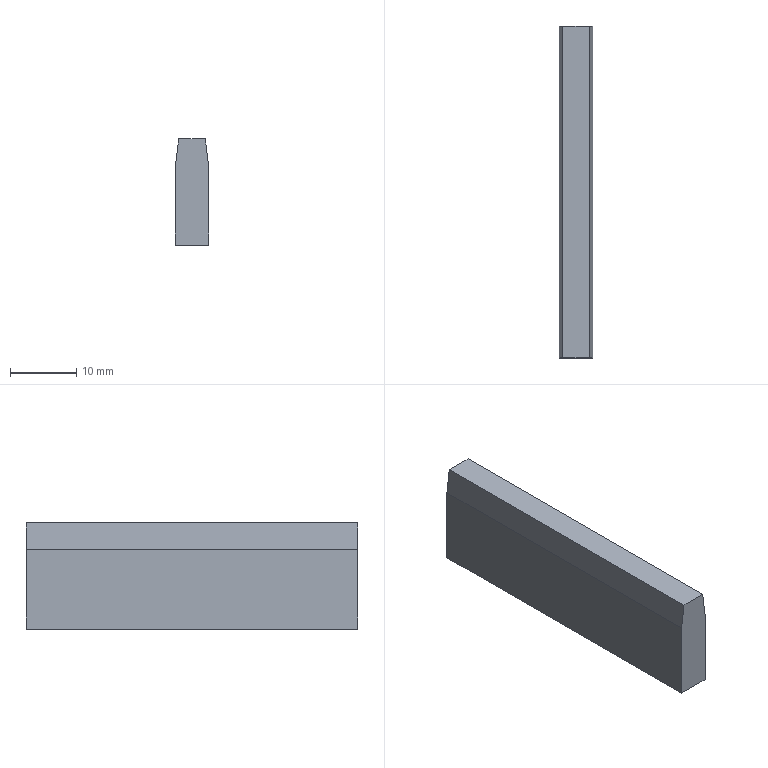Part | NX | features DATUM_CSYS 2, EXTRUDE 1, SKETCH 1 | 1 solid | 8 faces | box 5 x 50 x 16 mm | volume 3900 mm3 | plane 8
STEP:
#1=CARTESIAN_POINT('',(-2.5,0.,12.));
#2=VERTEX_POINT('',#1);
#3=CARTESIAN_POINT('',(-2.5,0.,0.));
#4=VERTEX_POINT('',#3);
#5=CARTESIAN_POINT('',(-2.5,0.,12.));
#6=DIRECTION('',(0.,0.,-1.));
#7=VECTOR('',#6,1000.);
#8=LINE('',#5,#7);
#9=EDGE_CURVE('',#2,#4,#8,.T.);
#10=ORIENTED_EDGE('',*,*,#9,.T.);
#11=CARTESIAN_POINT('',(-2.5,-50.,0.));
#12=VERTEX_POINT('',#11);
#13=CARTESIAN_POINT('',(-2.5,-50.,0.));
#14=DIRECTION('',(0.,1.,0.));
#15=VECTOR('',#14,1000.);
#16=LINE('',#13,#15);
#17=EDGE_CURVE('',#12,#4,#16,.T.);
#18=ORIENTED_EDGE('',*,*,#17,.F.);
#19=CARTESIAN_POINT('',(-2.5,-50.,12.));
#20=VERTEX_POINT('',#19);
#21=CARTESIAN_POINT('',(-2.5,-50.,12.));
#22=DIRECTION('',(0.,0.,-1.));
#23=VECTOR('',#22,1000.);
#24=LINE('',#21,#23);
#25=EDGE_CURVE('',#20,#12,#24,.T.);
#26=ORIENTED_EDGE('',*,*,#25,.F.);
#27=CARTESIAN_POINT('',(-2.5,-50.,12.));
#28=DIRECTION('',(0.,1.,0.));
#29=VECTOR('',#28,1000.);
#30=LINE('',#27,#29);
#31=EDGE_CURVE('',#20,#2,#30,.T.);
#32=ORIENTED_EDGE('',*,*,#31,.T.);
#33=EDGE_LOOP('',(#10,#18,#26,#32));
#34=FACE_BOUND('',#33,.T.);
#35=CARTESIAN_POINT('',(-2.5,-50.,12.));
#36=DIRECTION('',(1.,0.,0.));
#37=DIRECTION('',(0.,0.,-1.));
#38=AXIS2_PLACEMENT_3D('',#35,#36,#37);
#39=PLANE('',#38);
#40=ADVANCED_FACE('',(#34),#39,.F.);
#41=CARTESIAN_POINT('',(2.5,0.,0.));
#42=VERTEX_POINT('',#41);
#43=CARTESIAN_POINT('',(-2.5,0.,0.));
#44=DIRECTION('',(1.,0.,0.));
#45=VECTOR('',#44,1000.);
#46=LINE('',#43,#45);
#47=EDGE_CURVE('',#4,#42,#46,.T.);
#48=ORIENTED_EDGE('',*,*,#47,.T.);
#49=CARTESIAN_POINT('',(2.5,-50.,0.));
#50=VERTEX_POINT('',#49);
#51=CARTESIAN_POINT('',(2.5,-50.,0.));
#52=DIRECTION('',(0.,1.,0.));
#53=VECTOR('',#52,1000.);
#54=LINE('',#51,#53);
#55=EDGE_CURVE('',#50,#42,#54,.T.);
#56=ORIENTED_EDGE('',*,*,#55,.F.);
#57=CARTESIAN_POINT('',(-2.5,-50.,0.));
#58=DIRECTION('',(1.,0.,0.));
#59=VECTOR('',#58,1000.);
#60=LINE('',#57,#59);
#61=EDGE_CURVE('',#12,#50,#60,.T.);
#62=ORIENTED_EDGE('',*,*,#61,.F.);
#63=ORIENTED_EDGE('',*,*,#17,.T.);
#64=EDGE_LOOP('',(#48,#56,#62,#63));
#65=FACE_BOUND('',#64,.T.);
#66=CARTESIAN_POINT('',(-2.5,-50.,0.));
#67=DIRECTION('',(0.,0.,1.));
#68=DIRECTION('',(1.,0.,0.));
#69=AXIS2_PLACEMENT_3D('',#66,#67,#68);
#70=PLANE('',#69);
#71=ADVANCED_FACE('',(#65),#70,.F.);
#72=CARTESIAN_POINT('',(2.5,0.,12.));
#73=VERTEX_POINT('',#72);
#74=CARTESIAN_POINT('',(2.5,0.,0.));
#75=DIRECTION('',(0.,0.,1.));
#76=VECTOR('',#75,1000.);
#77=LINE('',#74,#76);
#78=EDGE_CURVE('',#42,#73,#77,.T.);
#79=ORIENTED_EDGE('',*,*,#78,.T.);
#80=CARTESIAN_POINT('',(2.5,-50.,12.));
#81=VERTEX_POINT('',#80);
#82=CARTESIAN_POINT('',(2.5,-50.,12.));
#83=DIRECTION('',(0.,1.,0.));
#84=VECTOR('',#83,1000.);
#85=LINE('',#82,#84);
#86=EDGE_CURVE('',#81,#73,#85,.T.);
#87=ORIENTED_EDGE('',*,*,#86,.F.);
#88=CARTESIAN_POINT('',(2.5,-50.,0.));
#89=DIRECTION('',(0.,0.,1.));
#90=VECTOR('',#89,1000.);
#91=LINE('',#88,#90);
#92=EDGE_CURVE('',#50,#81,#91,.T.);
#93=ORIENTED_EDGE('',*,*,#92,.F.);
#94=ORIENTED_EDGE('',*,*,#55,.T.);
#95=EDGE_LOOP('',(#79,#87,#93,#94));
#96=FACE_BOUND('',#95,.T.);
#97=CARTESIAN_POINT('',(2.5,-50.,0.));
#98=DIRECTION('',(-1.,0.,0.));
#99=DIRECTION('',(0.,0.,1.));
#100=AXIS2_PLACEMENT_3D('',#97,#98,#99);
#101=PLANE('',#100);
#102=ADVANCED_FACE('',(#96),#101,.F.);
#103=CARTESIAN_POINT('',(2.,0.,16.));
#104=VERTEX_POINT('',#103);
#105=CARTESIAN_POINT('',(2.5,0.,12.));
#106=DIRECTION('',(-0.124,0.,0.9923));
#107=VECTOR('',#106,1000.);
#108=LINE('',#105,#107);
#109=EDGE_CURVE('',#73,#104,#108,.T.);
#110=ORIENTED_EDGE('',*,*,#109,.T.);
#111=CARTESIAN_POINT('',(2.,-50.,16.));
#112=VERTEX_POINT('',#111);
#113=CARTESIAN_POINT('',(2.,-50.,16.));
#114=DIRECTION('',(0.,1.,0.));
#115=VECTOR('',#114,1000.);
#116=LINE('',#113,#115);
#117=EDGE_CURVE('',#112,#104,#116,.T.);
#118=ORIENTED_EDGE('',*,*,#117,.F.);
#119=CARTESIAN_POINT('',(2.5,-50.,12.));
#120=DIRECTION('',(-0.124,0.,0.9923));
#121=VECTOR('',#120,1000.);
#122=LINE('',#119,#121);
#123=EDGE_CURVE('',#81,#112,#122,.T.);
#124=ORIENTED_EDGE('',*,*,#123,.F.);
#125=ORIENTED_EDGE('',*,*,#86,.T.);
#126=EDGE_LOOP('',(#110,#118,#124,#125));
#127=FACE_BOUND('',#126,.T.);
#128=CARTESIAN_POINT('',(2.5,-50.,12.));
#129=DIRECTION('',(-0.9923,0.,-0.124));
#130=DIRECTION('',(-0.124,0.,0.9923));
#131=AXIS2_PLACEMENT_3D('',#128,#129,#130);
#132=PLANE('',#131);
#133=ADVANCED_FACE('',(#127),#132,.F.);
#134=CARTESIAN_POINT('',(-2.,0.,16.));
#135=VERTEX_POINT('',#134);
#136=CARTESIAN_POINT('',(2.,0.,16.));
#137=DIRECTION('',(-1.,0.,0.));
#138=VECTOR('',#137,1000.);
#139=LINE('',#136,#138);
#140=EDGE_CURVE('',#104,#135,#139,.T.);
#141=ORIENTED_EDGE('',*,*,#140,.T.);
#142=CARTESIAN_POINT('',(-2.,-50.,16.));
#143=VERTEX_POINT('',#142);
#144=CARTESIAN_POINT('',(-2.,-50.,16.));
#145=DIRECTION('',(0.,1.,0.));
#146=VECTOR('',#145,1000.);
#147=LINE('',#144,#146);
#148=EDGE_CURVE('',#143,#135,#147,.T.);
#149=ORIENTED_EDGE('',*,*,#148,.F.);
#150=CARTESIAN_POINT('',(2.,-50.,16.));
#151=DIRECTION('',(-1.,0.,0.));
#152=VECTOR('',#151,1000.);
#153=LINE('',#150,#152);
#154=EDGE_CURVE('',#112,#143,#153,.T.);
#155=ORIENTED_EDGE('',*,*,#154,.F.);
#156=ORIENTED_EDGE('',*,*,#117,.T.);
#157=EDGE_LOOP('',(#141,#149,#155,#156));
#158=FACE_BOUND('',#157,.T.);
#159=CARTESIAN_POINT('',(2.,-50.,16.));
#160=DIRECTION('',(0.,0.,-1.));
#161=DIRECTION('',(-1.,0.,0.));
#162=AXIS2_PLACEMENT_3D('',#159,#160,#161);
#163=PLANE('',#162);
#164=ADVANCED_FACE('',(#158),#163,.F.);
#165=CARTESIAN_POINT('',(-2.,0.,16.));
#166=DIRECTION('',(-0.124,0.,-0.9923));
#167=VECTOR('',#166,1000.);
#168=LINE('',#165,#167);
#169=EDGE_CURVE('',#135,#2,#168,.T.);
#170=ORIENTED_EDGE('',*,*,#169,.T.);
#171=ORIENTED_EDGE('',*,*,#31,.F.);
#172=CARTESIAN_POINT('',(-2.,-50.,16.));
#173=DIRECTION('',(-0.124,0.,-0.9923));
#174=VECTOR('',#173,1000.);
#175=LINE('',#172,#174);
#176=EDGE_CURVE('',#143,#20,#175,.T.);
#177=ORIENTED_EDGE('',*,*,#176,.F.);
#178=ORIENTED_EDGE('',*,*,#148,.T.);
#179=EDGE_LOOP('',(#170,#171,#177,#178));
#180=FACE_BOUND('',#179,.T.);
#181=CARTESIAN_POINT('',(-2.,-50.,16.));
#182=DIRECTION('',(0.9923,0.,-0.124));
#183=DIRECTION('',(-0.124,0.,-0.9923));
#184=AXIS2_PLACEMENT_3D('',#181,#182,#183);
#185=PLANE('',#184);
#186=ADVANCED_FACE('',(#180),#185,.F.);
#187=ORIENTED_EDGE('',*,*,#25,.T.);
#188=ORIENTED_EDGE('',*,*,#61,.T.);
#189=ORIENTED_EDGE('',*,*,#92,.T.);
#190=ORIENTED_EDGE('',*,*,#123,.T.);
#191=ORIENTED_EDGE('',*,*,#154,.T.);
#192=ORIENTED_EDGE('',*,*,#176,.T.);
#193=EDGE_LOOP('',(#187,#188,#189,#190,#191,#192));
#194=FACE_BOUND('',#193,.T.);
#195=CARTESIAN_POINT('',(0.,-50.,0.));
#196=DIRECTION('',(0.,-1.,0.));
#197=DIRECTION('',(0.,0.,-1.));
#198=AXIS2_PLACEMENT_3D('',#195,#196,#197);
#199=PLANE('',#198);
#200=ADVANCED_FACE('',(#194),#199,.T.);
#201=ORIENTED_EDGE('',*,*,#9,.F.);
#202=ORIENTED_EDGE('',*,*,#169,.F.);
#203=ORIENTED_EDGE('',*,*,#140,.F.);
#204=ORIENTED_EDGE('',*,*,#109,.F.);
#205=ORIENTED_EDGE('',*,*,#78,.F.);
#206=ORIENTED_EDGE('',*,*,#47,.F.);
#207=EDGE_LOOP('',(#201,#202,#203,#204,#205,#206));
#208=FACE_BOUND('',#207,.T.);
#209=CARTESIAN_POINT('',(0.,0.,0.));
#210=DIRECTION('',(0.,-1.,0.));
#211=DIRECTION('',(0.,0.,-1.));
#212=AXIS2_PLACEMENT_3D('',#209,#210,#211);
#213=PLANE('',#212);
#214=ADVANCED_FACE('',(#208),#213,.F.);
#215=CLOSED_SHELL('',(#40,#71,#102,#133,#164,#186,#200,#214));
#216=MANIFOLD_SOLID_BREP('',#215);
#217=(LENGTH_UNIT()NAMED_UNIT(*)SI_UNIT(.MILLI.,.METRE.));
#218=UNCERTAINTY_MEASURE_WITH_UNIT(LENGTH_MEASURE(0.00001),#217,'','');
#219=(NAMED_UNIT(*)PLANE_ANGLE_UNIT()SI_UNIT($,.RADIAN.));
#220=(NAMED_UNIT(*)SI_UNIT($,.STERADIAN.)SOLID_ANGLE_UNIT());
#221=(GEOMETRIC_REPRESENTATION_CONTEXT(3)GLOBAL_UNCERTAINTY_ASSIGNED_CONTEXT((#218))GLOBAL_UNIT_ASSIGNED_CONTEXT((#217,#219,#220))REPRESENTATION_CONTEXT('',''));
#222=ADVANCED_BREP_SHAPE_REPRESENTATION('',(#216),#221);